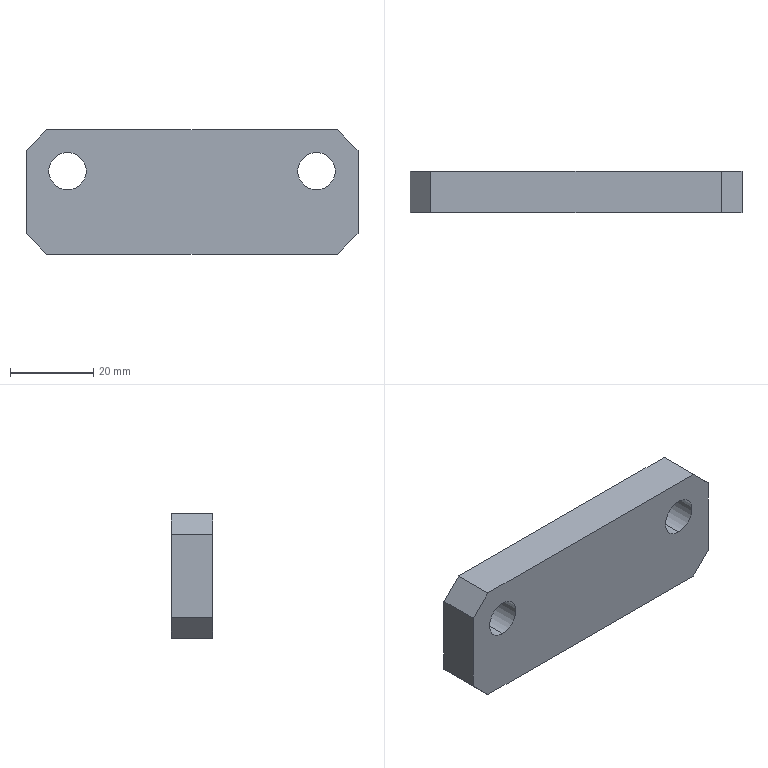Part | SolidWorks | features BaseBody 1 | 1 solid | 28 faces | box 80 x 10 x 30 mm | volume 21712 mm3 | cylinder 12 | plane 12 | cone 4 | commonest cylinder face diameters 4.2 x4 5 x4 9 x4
STEP:
#1=CARTESIAN_POINT('',(-30.,0.,0.5));
#2=VERTEX_POINT('',#1);
#3=CARTESIAN_POINT('',(-30.,0.,9.5));
#4=VERTEX_POINT('',#3);
#5=CARTESIAN_POINT('',(-30.,0.,5.));
#6=DIRECTION('',(0.,1.,0.));
#7=DIRECTION('',(0.,0.,1.));
#8=AXIS2_PLACEMENT_3D('',#5,#6,#7);
#9=CIRCLE('',#8,4.5);
#10=EDGE_CURVE('',#2,#4,#9,.T.);
#11=ORIENTED_EDGE('',*,*,#10,.F.);
#12=CARTESIAN_POINT('',(-30.,10.,0.5));
#13=VERTEX_POINT('',#12);
#14=CARTESIAN_POINT('',(-30.,10.,0.5));
#15=DIRECTION('',(0.,1.,0.));
#16=VECTOR('',#15,1000.);
#17=LINE('',#14,#16);
#18=EDGE_CURVE('',#2,#13,#17,.T.);
#19=ORIENTED_EDGE('',*,*,#18,.T.);
#20=CARTESIAN_POINT('',(-30.,10.,9.5));
#21=VERTEX_POINT('',#20);
#22=CARTESIAN_POINT('',(-30.,10.,5.));
#23=DIRECTION('',(0.,1.,0.));
#24=DIRECTION('',(0.,0.,1.));
#25=AXIS2_PLACEMENT_3D('',#22,#23,#24);
#26=CIRCLE('',#25,4.5);
#27=EDGE_CURVE('',#13,#21,#26,.T.);
#28=ORIENTED_EDGE('',*,*,#27,.T.);
#29=CARTESIAN_POINT('',(-30.,10.,9.5));
#30=DIRECTION('',(0.,1.,0.));
#31=VECTOR('',#30,1000.);
#32=LINE('',#29,#31);
#33=EDGE_CURVE('',#4,#21,#32,.T.);
#34=ORIENTED_EDGE('',*,*,#33,.F.);
#35=EDGE_LOOP('',(#11,#19,#28,#34));
#36=FACE_OUTER_BOUND('',#35,.T.);
#37=CARTESIAN_POINT('',(-30.,10.,5.));
#38=DIRECTION('',(0.,1.,0.));
#39=DIRECTION('',(0.,0.,1.));
#40=AXIS2_PLACEMENT_3D('',#37,#38,#39);
#41=CYLINDRICAL_SURFACE('',#40,4.5);
#42=ADVANCED_FACE('',(#36),#41,.F.);
#43=CARTESIAN_POINT('',(30.,0.,0.5));
#44=VERTEX_POINT('',#43);
#45=CARTESIAN_POINT('',(30.,0.,9.5));
#46=VERTEX_POINT('',#45);
#47=CARTESIAN_POINT('',(30.,0.,5.));
#48=DIRECTION('',(0.,1.,0.));
#49=DIRECTION('',(0.,0.,1.));
#50=AXIS2_PLACEMENT_3D('',#47,#48,#49);
#51=CIRCLE('',#50,4.5);
#52=EDGE_CURVE('',#44,#46,#51,.T.);
#53=ORIENTED_EDGE('',*,*,#52,.F.);
#54=CARTESIAN_POINT('',(30.,10.,0.5));
#55=VERTEX_POINT('',#54);
#56=CARTESIAN_POINT('',(30.,10.,0.5));
#57=DIRECTION('',(0.,1.,0.));
#58=VECTOR('',#57,1000.);
#59=LINE('',#56,#58);
#60=EDGE_CURVE('',#44,#55,#59,.T.);
#61=ORIENTED_EDGE('',*,*,#60,.T.);
#62=CARTESIAN_POINT('',(30.,10.,9.5));
#63=VERTEX_POINT('',#62);
#64=CARTESIAN_POINT('',(30.,10.,5.));
#65=DIRECTION('',(0.,1.,0.));
#66=DIRECTION('',(0.,0.,1.));
#67=AXIS2_PLACEMENT_3D('',#64,#65,#66);
#68=CIRCLE('',#67,4.5);
#69=EDGE_CURVE('',#55,#63,#68,.T.);
#70=ORIENTED_EDGE('',*,*,#69,.T.);
#71=CARTESIAN_POINT('',(30.,10.,9.5));
#72=DIRECTION('',(0.,1.,0.));
#73=VECTOR('',#72,1000.);
#74=LINE('',#71,#73);
#75=EDGE_CURVE('',#46,#63,#74,.T.);
#76=ORIENTED_EDGE('',*,*,#75,.F.);
#77=EDGE_LOOP('',(#53,#61,#70,#76));
#78=FACE_OUTER_BOUND('',#77,.T.);
#79=CARTESIAN_POINT('',(30.,10.,5.));
#80=DIRECTION('',(0.,1.,0.));
#81=DIRECTION('',(0.,0.,1.));
#82=AXIS2_PLACEMENT_3D('',#79,#80,#81);
#83=CYLINDRICAL_SURFACE('',#82,4.5);
#84=ADVANCED_FACE('',(#78),#83,.F.);
#85=CARTESIAN_POINT('',(17.5,5.,-5.));
#86=VERTEX_POINT('',#85);
#87=CARTESIAN_POINT('',(12.5,5.,-5.));
#88=VERTEX_POINT('',#87);
#89=CARTESIAN_POINT('',(15.,5.,-5.));
#90=DIRECTION('',(0.,0.,-1.));
#91=DIRECTION('',(-1.,0.,0.));
#92=AXIS2_PLACEMENT_3D('',#89,#90,#91);
#93=CIRCLE('',#92,2.5);
#94=EDGE_CURVE('',#86,#88,#93,.T.);
#95=ORIENTED_EDGE('',*,*,#94,.F.);
#96=CARTESIAN_POINT('',(17.5,5.,-15.));
#97=VERTEX_POINT('',#96);
#98=CARTESIAN_POINT('',(17.5,5.,-15.));
#99=DIRECTION('',(0.,0.,-1.));
#100=VECTOR('',#99,1000.);
#101=LINE('',#98,#100);
#102=EDGE_CURVE('',#86,#97,#101,.T.);
#103=ORIENTED_EDGE('',*,*,#102,.T.);
#104=CARTESIAN_POINT('',(12.5,5.,-15.));
#105=VERTEX_POINT('',#104);
#106=CARTESIAN_POINT('',(15.,5.,-15.));
#107=DIRECTION('',(0.,0.,-1.));
#108=DIRECTION('',(-1.,0.,0.));
#109=AXIS2_PLACEMENT_3D('',#106,#107,#108);
#110=CIRCLE('',#109,2.5);
#111=EDGE_CURVE('',#97,#105,#110,.T.);
#112=ORIENTED_EDGE('',*,*,#111,.T.);
#113=CARTESIAN_POINT('',(12.5,5.,-15.));
#114=DIRECTION('',(0.,0.,-1.));
#115=VECTOR('',#114,1000.);
#116=LINE('',#113,#115);
#117=EDGE_CURVE('',#88,#105,#116,.T.);
#118=ORIENTED_EDGE('',*,*,#117,.F.);
#119=EDGE_LOOP('',(#95,#103,#112,#118));
#120=FACE_OUTER_BOUND('',#119,.T.);
#121=CARTESIAN_POINT('',(15.,5.,-15.));
#122=DIRECTION('',(0.,0.,-1.));
#123=DIRECTION('',(-1.,0.,0.));
#124=AXIS2_PLACEMENT_3D('',#121,#122,#123);
#125=CYLINDRICAL_SURFACE('',#124,2.5);
#126=ADVANCED_FACE('',(#120),#125,.F.);
#127=CARTESIAN_POINT('',(17.1,5.,-1.));
#128=VERTEX_POINT('',#127);
#129=CARTESIAN_POINT('',(12.9,5.,-1.));
#130=VERTEX_POINT('',#129);
#131=CARTESIAN_POINT('',(15.,5.,-1.));
#132=DIRECTION('',(0.,0.,-1.));
#133=DIRECTION('',(-1.,0.,0.));
#134=AXIS2_PLACEMENT_3D('',#131,#132,#133);
#135=CIRCLE('',#134,2.1);
#136=EDGE_CURVE('',#128,#130,#135,.T.);
#137=ORIENTED_EDGE('',*,*,#136,.F.);
#138=CARTESIAN_POINT('',(17.1,5.,-5.));
#139=VERTEX_POINT('',#138);
#140=CARTESIAN_POINT('',(17.1,5.,-15.));
#141=DIRECTION('',(0.,0.,-1.));
#142=VECTOR('',#141,1000.);
#143=LINE('',#140,#142);
#144=EDGE_CURVE('',#128,#139,#143,.T.);
#145=ORIENTED_EDGE('',*,*,#144,.T.);
#146=CARTESIAN_POINT('',(12.9,5.,-5.));
#147=VERTEX_POINT('',#146);
#148=CARTESIAN_POINT('',(15.,5.,-5.));
#149=DIRECTION('',(0.,0.,-1.));
#150=DIRECTION('',(-1.,0.,0.));
#151=AXIS2_PLACEMENT_3D('',#148,#149,#150);
#152=CIRCLE('',#151,2.1);
#153=EDGE_CURVE('',#139,#147,#152,.T.);
#154=ORIENTED_EDGE('',*,*,#153,.T.);
#155=CARTESIAN_POINT('',(12.9,5.,-15.));
#156=DIRECTION('',(0.,0.,-1.));
#157=VECTOR('',#156,1000.);
#158=LINE('',#155,#157);
#159=EDGE_CURVE('',#130,#147,#158,.T.);
#160=ORIENTED_EDGE('',*,*,#159,.F.);
#161=EDGE_LOOP('',(#137,#145,#154,#160));
#162=FACE_OUTER_BOUND('',#161,.T.);
#163=CARTESIAN_POINT('',(15.,5.,-15.));
#164=DIRECTION('',(0.,0.,-1.));
#165=DIRECTION('',(-1.,0.,0.));
#166=AXIS2_PLACEMENT_3D('',#163,#164,#165);
#167=CYLINDRICAL_SURFACE('',#166,2.1);
#168=ADVANCED_FACE('',(#162),#167,.F.);
#169=CARTESIAN_POINT('',(15.,5.,0.2618));
#170=VERTEX_POINT('',#169);
#171=CARTESIAN_POINT('',(12.9,5.,-1.));
#172=DIRECTION('',(-0.8572,0.,-0.515));
#173=VECTOR('',#172,1000.);
#174=LINE('',#171,#173);
#175=EDGE_CURVE('',#170,#130,#174,.T.);
#176=ORIENTED_EDGE('',*,*,#175,.F.);
#177=CARTESIAN_POINT('',(17.1,5.,-1.));
#178=DIRECTION('',(0.8572,0.,-0.515));
#179=VECTOR('',#178,1000.);
#180=LINE('',#177,#179);
#181=EDGE_CURVE('',#170,#128,#180,.T.);
#182=ORIENTED_EDGE('',*,*,#181,.T.);
#183=ORIENTED_EDGE('',*,*,#136,.T.);
#184=EDGE_LOOP('',(#176,#182,#183));
#185=FACE_OUTER_BOUND('',#184,.T.);
#186=CARTESIAN_POINT('',(15.,5.,-1.));
#187=DIRECTION('',(0.,0.,-1.));
#188=DIRECTION('',(-1.,0.,0.));
#189=AXIS2_PLACEMENT_3D('',#186,#187,#188);
#190=CONICAL_SURFACE('',#189,2.1,1.03);
#191=ADVANCED_FACE('',(#185),#190,.F.);
#192=CARTESIAN_POINT('',(-12.5,5.,-5.));
#193=VERTEX_POINT('',#192);
#194=CARTESIAN_POINT('',(-17.5,5.,-5.));
#195=VERTEX_POINT('',#194);
#196=CARTESIAN_POINT('',(-15.,5.,-5.));
#197=DIRECTION('',(0.,0.,-1.));
#198=DIRECTION('',(-1.,0.,0.));
#199=AXIS2_PLACEMENT_3D('',#196,#197,#198);
#200=CIRCLE('',#199,2.5);
#201=EDGE_CURVE('',#193,#195,#200,.T.);
#202=ORIENTED_EDGE('',*,*,#201,.F.);
#203=CARTESIAN_POINT('',(-12.5,5.,-15.));
#204=VERTEX_POINT('',#203);
#205=CARTESIAN_POINT('',(-12.5,5.,-15.));
#206=DIRECTION('',(0.,0.,-1.));
#207=VECTOR('',#206,1000.);
#208=LINE('',#205,#207);
#209=EDGE_CURVE('',#193,#204,#208,.T.);
#210=ORIENTED_EDGE('',*,*,#209,.T.);
#211=CARTESIAN_POINT('',(-17.5,5.,-15.));
#212=VERTEX_POINT('',#211);
#213=CARTESIAN_POINT('',(-15.,5.,-15.));
#214=DIRECTION('',(0.,0.,-1.));
#215=DIRECTION('',(-1.,0.,0.));
#216=AXIS2_PLACEMENT_3D('',#213,#214,#215);
#217=CIRCLE('',#216,2.5);
#218=EDGE_CURVE('',#204,#212,#217,.T.);
#219=ORIENTED_EDGE('',*,*,#218,.T.);
#220=CARTESIAN_POINT('',(-17.5,5.,-15.));
#221=DIRECTION('',(0.,0.,-1.));
#222=VECTOR('',#221,1000.);
#223=LINE('',#220,#222);
#224=EDGE_CURVE('',#195,#212,#223,.T.);
#225=ORIENTED_EDGE('',*,*,#224,.F.);
#226=EDGE_LOOP('',(#202,#210,#219,#225));
#227=FACE_OUTER_BOUND('',#226,.T.);
#228=CARTESIAN_POINT('',(-15.,5.,-15.));
#229=DIRECTION('',(0.,0.,-1.));
#230=DIRECTION('',(-1.,0.,0.));
#231=AXIS2_PLACEMENT_3D('',#228,#229,#230);
#232=CYLINDRICAL_SURFACE('',#231,2.5);
#233=ADVANCED_FACE('',(#227),#232,.F.);
#234=CARTESIAN_POINT('',(-12.9,5.,-1.));
#235=VERTEX_POINT('',#234);
#236=CARTESIAN_POINT('',(-17.1,5.,-1.));
#237=VERTEX_POINT('',#236);
#238=CARTESIAN_POINT('',(-15.,5.,-1.));
#239=DIRECTION('',(0.,0.,-1.));
#240=DIRECTION('',(-1.,0.,0.));
#241=AXIS2_PLACEMENT_3D('',#238,#239,#240);
#242=CIRCLE('',#241,2.1);
#243=EDGE_CURVE('',#235,#237,#242,.T.);
#244=ORIENTED_EDGE('',*,*,#243,.F.);
#245=CARTESIAN_POINT('',(-12.9,5.,-5.));
#246=VERTEX_POINT('',#245);
#247=CARTESIAN_POINT('',(-12.9,5.,-15.));
#248=DIRECTION('',(0.,0.,-1.));
#249=VECTOR('',#248,1000.);
#250=LINE('',#247,#249);
#251=EDGE_CURVE('',#235,#246,#250,.T.);
#252=ORIENTED_EDGE('',*,*,#251,.T.);
#253=CARTESIAN_POINT('',(-17.1,5.,-5.));
#254=VERTEX_POINT('',#253);
#255=CARTESIAN_POINT('',(-15.,5.,-5.));
#256=DIRECTION('',(0.,0.,-1.));
#257=DIRECTION('',(-1.,0.,0.));
#258=AXIS2_PLACEMENT_3D('',#255,#256,#257);
#259=CIRCLE('',#258,2.1);
#260=EDGE_CURVE('',#246,#254,#259,.T.);
#261=ORIENTED_EDGE('',*,*,#260,.T.);
#262=CARTESIAN_POINT('',(-17.1,5.,-15.));
#263=DIRECTION('',(0.,0.,-1.));
#264=VECTOR('',#263,1000.);
#265=LINE('',#262,#264);
#266=EDGE_CURVE('',#237,#254,#265,.T.);
#267=ORIENTED_EDGE('',*,*,#266,.F.);
#268=EDGE_LOOP('',(#244,#252,#261,#267));
#269=FACE_OUTER_BOUND('',#268,.T.);
#270=CARTESIAN_POINT('',(-15.,5.,-15.));
#271=DIRECTION('',(0.,0.,-1.));
#272=DIRECTION('',(-1.,0.,0.));
#273=AXIS2_PLACEMENT_3D('',#270,#271,#272);
#274=CYLINDRICAL_SURFACE('',#273,2.1);
#275=ADVANCED_FACE('',(#269),#274,.F.);
#276=CARTESIAN_POINT('',(-15.,5.,0.2618));
#277=VERTEX_POINT('',#276);
#278=CARTESIAN_POINT('',(-17.1,5.,-1.));
#279=DIRECTION('',(-0.8572,0.,-0.515));
#280=VECTOR('',#279,1000.);
#281=LINE('',#278,#280);
#282=EDGE_CURVE('',#277,#237,#281,.T.);
#283=ORIENTED_EDGE('',*,*,#282,.F.);
#284=CARTESIAN_POINT('',(-12.9,5.,-1.));
#285=DIRECTION('',(0.8572,0.,-0.515));
#286=VECTOR('',#285,1000.);
#287=LINE('',#284,#286);
#288=EDGE_CURVE('',#277,#235,#287,.T.);
#289=ORIENTED_EDGE('',*,*,#288,.T.);
#290=ORIENTED_EDGE('',*,*,#243,.T.);
#291=EDGE_LOOP('',(#283,#289,#290));
#292=FACE_OUTER_BOUND('',#291,.T.);
#293=CARTESIAN_POINT('',(-15.,5.,-1.));
#294=DIRECTION('',(0.,0.,-1.));
#295=DIRECTION('',(-1.,0.,0.));
#296=AXIS2_PLACEMENT_3D('',#293,#294,#295);
#297=CONICAL_SURFACE('',#296,2.1,1.03);
#298=ADVANCED_FACE('',(#292),#297,.F.);
#299=CARTESIAN_POINT('',(-40.,0.,-10.));
#300=VERTEX_POINT('',#299);
#301=CARTESIAN_POINT('',(-40.,0.,10.));
#302=VERTEX_POINT('',#301);
#303=CARTESIAN_POINT('',(-40.,0.,-15.));
#304=DIRECTION('',(0.,0.,1.));
#305=VECTOR('',#304,1000.);
#306=LINE('',#303,#305);
#307=EDGE_CURVE('',#300,#302,#306,.T.);
#308=ORIENTED_EDGE('',*,*,#307,.T.);
#309=CARTESIAN_POINT('',(-40.,10.,10.));
#310=VERTEX_POINT('',#309);
#311=CARTESIAN_POINT('',(-40.,10.,10.));
#312=DIRECTION('',(0.,1.,0.));
#313=VECTOR('',#312,1000.);
#314=LINE('',#311,#313);
#315=EDGE_CURVE('',#302,#310,#314,.T.);
#316=ORIENTED_EDGE('',*,*,#315,.T.);
#317=CARTESIAN_POINT('',(-40.,10.,-10.));
#318=VERTEX_POINT('',#317);
#319=CARTESIAN_POINT('',(-40.,10.,-15.));
#320=DIRECTION('',(0.,0.,1.));
#321=VECTOR('',#320,1000.);
#322=LINE('',#319,#321);
#323=EDGE_CURVE('',#318,#310,#322,.T.);
#324=ORIENTED_EDGE('',*,*,#323,.F.);
#325=CARTESIAN_POINT('',(-40.,10.,-10.));
#326=DIRECTION('',(0.,-1.,0.));
#327=VECTOR('',#326,1000.);
#328=LINE('',#325,#327);
#329=EDGE_CURVE('',#318,#300,#328,.T.);
#330=ORIENTED_EDGE('',*,*,#329,.T.);
#331=EDGE_LOOP('',(#308,#316,#324,#330));
#332=FACE_OUTER_BOUND('',#331,.T.);
#333=CARTESIAN_POINT('',(-40.,10.,-15.));
#334=DIRECTION('',(1.,0.,0.));
#335=DIRECTION('',(0.,0.,-1.));
#336=AXIS2_PLACEMENT_3D('',#333,#334,#335);
#337=PLANE('',#336);
#338=ADVANCED_FACE('',(#332),#337,.F.);
#339=CARTESIAN_POINT('',(-35.,0.,15.));
#340=VERTEX_POINT('',#339);
#341=CARTESIAN_POINT('',(35.,0.,15.));
#342=VERTEX_POINT('',#341);
#343=CARTESIAN_POINT('',(40.,0.,15.));
#344=DIRECTION('',(1.,0.,0.));
#345=VECTOR('',#344,1000.);
#346=LINE('',#343,#345);
#347=EDGE_CURVE('',#340,#342,#346,.T.);
#348=ORIENTED_EDGE('',*,*,#347,.T.);
#349=CARTESIAN_POINT('',(35.,10.,15.));
#350=VERTEX_POINT('',#349);
#351=CARTESIAN_POINT('',(35.,10.,15.));
#352=DIRECTION('',(0.,1.,0.));
#353=VECTOR('',#352,1000.);
#354=LINE('',#351,#353);
#355=EDGE_CURVE('',#342,#350,#354,.T.);
#356=ORIENTED_EDGE('',*,*,#355,.T.);
#357=CARTESIAN_POINT('',(-35.,10.,15.));
#358=VERTEX_POINT('',#357);
#359=CARTESIAN_POINT('',(40.,10.,15.));
#360=DIRECTION('',(1.,0.,0.));
#361=VECTOR('',#360,1000.);
#362=LINE('',#359,#361);
#363=EDGE_CURVE('',#358,#350,#362,.T.);
#364=ORIENTED_EDGE('',*,*,#363,.F.);
#365=CARTESIAN_POINT('',(-35.,10.,15.));
#366=DIRECTION('',(0.,-1.,0.));
#367=VECTOR('',#366,1000.);
#368=LINE('',#365,#367);
#369=EDGE_CURVE('',#358,#340,#368,.T.);
#370=ORIENTED_EDGE('',*,*,#369,.T.);
#371=EDGE_LOOP('',(#348,#356,#364,#370));
#372=FACE_OUTER_BOUND('',#371,.T.);
#373=CARTESIAN_POINT('',(40.,10.,15.));
#374=DIRECTION('',(0.,0.,-1.));
#375=DIRECTION('',(-1.,0.,0.));
#376=AXIS2_PLACEMENT_3D('',#373,#374,#375);
#377=PLANE('',#376);
#378=ADVANCED_FACE('',(#372),#377,.F.);
#379=CARTESIAN_POINT('',(40.,0.,10.));
#380=VERTEX_POINT('',#379);
#381=CARTESIAN_POINT('',(40.,0.,-10.));
#382=VERTEX_POINT('',#381);
#383=CARTESIAN_POINT('',(40.,0.,-15.));
#384=DIRECTION('',(0.,0.,-1.));
#385=VECTOR('',#384,1000.);
#386=LINE('',#383,#385);
#387=EDGE_CURVE('',#380,#382,#386,.T.);
#388=ORIENTED_EDGE('',*,*,#387,.T.);
#389=CARTESIAN_POINT('',(40.,10.,-10.));
#390=VERTEX_POINT('',#389);
#391=CARTESIAN_POINT('',(40.,10.,-10.));
#392=DIRECTION('',(0.,1.,0.));
#393=VECTOR('',#392,1000.);
#394=LINE('',#391,#393);
#395=EDGE_CURVE('',#382,#390,#394,.T.);
#396=ORIENTED_EDGE('',*,*,#395,.T.);
#397=CARTESIAN_POINT('',(40.,10.,10.));
#398=VERTEX_POINT('',#397);
#399=CARTESIAN_POINT('',(40.,10.,-15.));
#400=DIRECTION('',(0.,0.,-1.));
#401=VECTOR('',#400,1000.);
#402=LINE('',#399,#401);
#403=EDGE_CURVE('',#398,#390,#402,.T.);
#404=ORIENTED_EDGE('',*,*,#403,.F.);
#405=CARTESIAN_POINT('',(40.,10.,10.));
#406=DIRECTION('',(0.,-1.,0.));
#407=VECTOR('',#406,1000.);
#408=LINE('',#405,#407);
#409=EDGE_CURVE('',#398,#380,#408,.T.);
#410=ORIENTED_EDGE('',*,*,#409,.T.);
#411=EDGE_LOOP('',(#388,#396,#404,#410));
#412=FACE_OUTER_BOUND('',#411,.T.);
#413=CARTESIAN_POINT('',(40.,10.,-15.));
#414=DIRECTION('',(-1.,0.,0.));
#415=DIRECTION('',(0.,0.,1.));
#416=AXIS2_PLACEMENT_3D('',#413,#414,#415);
#417=PLANE('',#416);
#418=ADVANCED_FACE('',(#412),#417,.F.);
#419=CARTESIAN_POINT('',(15.,5.,-15.));
#420=DIRECTION('',(0.,0.,-1.));
#421=DIRECTION('',(-1.,0.,0.));
#422=AXIS2_PLACEMENT_3D('',#419,#420,#421);
#423=CIRCLE('',#422,2.5);
#424=EDGE_CURVE('',#105,#97,#423,.T.);
#425=ORIENTED_EDGE('',*,*,#424,.F.);
#426=ORIENTED_EDGE('',*,*,#111,.F.);
#427=EDGE_LOOP('',(#425,#426));
#428=FACE_BOUND('',#427,.T.);
#429=CARTESIAN_POINT('',(-15.,5.,-15.));
#430=DIRECTION('',(0.,0.,-1.));
#431=DIRECTION('',(-1.,0.,0.));
#432=AXIS2_PLACEMENT_3D('',#429,#430,#431);
#433=CIRCLE('',#432,2.5);
#434=EDGE_CURVE('',#212,#204,#433,.T.);
#435=ORIENTED_EDGE('',*,*,#434,.F.);
#436=ORIENTED_EDGE('',*,*,#218,.F.);
#437=EDGE_LOOP('',(#435,#436));
#438=FACE_BOUND('',#437,.T.);
#439=CARTESIAN_POINT('',(35.,10.,-15.));
#440=VERTEX_POINT('',#439);
#441=CARTESIAN_POINT('',(-35.,10.,-15.));
#442=VERTEX_POINT('',#441);
#443=CARTESIAN_POINT('',(40.,10.,-15.));
#444=DIRECTION('',(-1.,0.,0.));
#445=VECTOR('',#444,1000.);
#446=LINE('',#443,#445);
#447=EDGE_CURVE('',#440,#442,#446,.T.);
#448=ORIENTED_EDGE('',*,*,#447,.F.);
#449=CARTESIAN_POINT('',(35.,0.,-15.));
#450=VERTEX_POINT('',#449);
#451=CARTESIAN_POINT('',(35.,10.,-15.));
#452=DIRECTION('',(0.,-1.,0.));
#453=VECTOR('',#452,1000.);
#454=LINE('',#451,#453);
#455=EDGE_CURVE('',#440,#450,#454,.T.);
#456=ORIENTED_EDGE('',*,*,#455,.T.);
#457=CARTESIAN_POINT('',(-35.,0.,-15.));
#458=VERTEX_POINT('',#457);
#459=CARTESIAN_POINT('',(40.,0.,-15.));
#460=DIRECTION('',(-1.,0.,0.));
#461=VECTOR('',#460,1000.);
#462=LINE('',#459,#461);
#463=EDGE_CURVE('',#450,#458,#462,.T.);
#464=ORIENTED_EDGE('',*,*,#463,.T.);
#465=CARTESIAN_POINT('',(-35.,10.,-15.));
#466=DIRECTION('',(0.,1.,0.));
#467=VECTOR('',#466,1000.);
#468=LINE('',#465,#467);
#469=EDGE_CURVE('',#458,#442,#468,.T.);
#470=ORIENTED_EDGE('',*,*,#469,.T.);
#471=EDGE_LOOP('',(#448,#456,#464,#470));
#472=FACE_OUTER_BOUND('',#471,.T.);
#473=CARTESIAN_POINT('',(40.,10.,-15.));
#474=DIRECTION('',(0.,0.,1.));
#475=DIRECTION('',(1.,0.,0.));
#476=AXIS2_PLACEMENT_3D('',#473,#474,#475);
#477=PLANE('',#476);
#478=ADVANCED_FACE('',(#428,#438,#472),#477,.F.);
#479=CARTESIAN_POINT('',(-30.,10.,5.));
#480=DIRECTION('',(0.,1.,0.));
#481=DIRECTION('',(0.,0.,1.));
#482=AXIS2_PLACEMENT_3D('',#479,#480,#481);
#483=CIRCLE('',#482,4.5);
#484=EDGE_CURVE('',#21,#13,#483,.T.);
#485=ORIENTED_EDGE('',*,*,#484,.F.);
#486=ORIENTED_EDGE('',*,*,#27,.F.);
#487=EDGE_LOOP('',(#485,#486));
#488=FACE_BOUND('',#487,.T.);
#489=CARTESIAN_POINT('',(30.,10.,5.));
#490=DIRECTION('',(0.,1.,0.));
#491=DIRECTION('',(0.,0.,1.));
#492=AXIS2_PLACEMENT_3D('',#489,#490,#491);
#493=CIRCLE('',#492,4.5);
#494=EDGE_CURVE('',#63,#55,#493,.T.);
#495=ORIENTED_EDGE('',*,*,#494,.F.);
#496=ORIENTED_EDGE('',*,*,#69,.F.);
#497=EDGE_LOOP('',(#495,#496));
#498=FACE_BOUND('',#497,.T.);
#499=ORIENTED_EDGE('',*,*,#403,.T.);
#500=CARTESIAN_POINT('',(35.,10.,-15.));
#501=DIRECTION('',(-0.7071,0.,-0.7071));
#502=VECTOR('',#501,1000.);
#503=LINE('',#500,#502);
#504=EDGE_CURVE('',#390,#440,#503,.T.);
#505=ORIENTED_EDGE('',*,*,#504,.T.);
#506=ORIENTED_EDGE('',*,*,#447,.T.);
#507=CARTESIAN_POINT('',(-40.,10.,-10.));
#508=DIRECTION('',(-0.7071,0.,0.7071));
#509=VECTOR('',#508,1000.);
#510=LINE('',#507,#509);
#511=EDGE_CURVE('',#442,#318,#510,.T.);
#512=ORIENTED_EDGE('',*,*,#511,.T.);
#513=ORIENTED_EDGE('',*,*,#323,.T.);
#514=CARTESIAN_POINT('',(-35.,10.,15.));
#515=DIRECTION('',(0.7071,0.,0.7071));
#516=VECTOR('',#515,1000.);
#517=LINE('',#514,#516);
#518=EDGE_CURVE('',#310,#358,#517,.T.);
#519=ORIENTED_EDGE('',*,*,#518,.T.);
#520=ORIENTED_EDGE('',*,*,#363,.T.);
#521=CARTESIAN_POINT('',(40.,10.,10.));
#522=DIRECTION('',(0.7071,0.,-0.7071));
#523=VECTOR('',#522,1000.);
#524=LINE('',#521,#523);
#525=EDGE_CURVE('',#350,#398,#524,.T.);
#526=ORIENTED_EDGE('',*,*,#525,.T.);
#527=EDGE_LOOP('',(#499,#505,#506,#512,#513,#519,#520,#526));
#528=FACE_OUTER_BOUND('',#527,.T.);
#529=CARTESIAN_POINT('',(0.,10.,0.));
#530=DIRECTION('',(0.,-1.,0.));
#531=DIRECTION('',(0.,0.,-1.));
#532=AXIS2_PLACEMENT_3D('',#529,#530,#531);
#533=PLANE('',#532);
#534=ADVANCED_FACE('',(#488,#498,#528),#533,.F.);
#535=CARTESIAN_POINT('',(-30.,0.,5.));
#536=DIRECTION('',(0.,1.,0.));
#537=DIRECTION('',(0.,0.,1.));
#538=AXIS2_PLACEMENT_3D('',#535,#536,#537);
#539=CIRCLE('',#538,4.5);
#540=EDGE_CURVE('',#4,#2,#539,.T.);
#541=ORIENTED_EDGE('',*,*,#540,.T.);
#542=ORIENTED_EDGE('',*,*,#10,.T.);
#543=EDGE_LOOP('',(#541,#542));
#544=FACE_BOUND('',#543,.T.);
#545=CARTESIAN_POINT('',(30.,0.,5.));
#546=DIRECTION('',(0.,1.,0.));
#547=DIRECTION('',(0.,0.,1.));
#548=AXIS2_PLACEMENT_3D('',#545,#546,#547);
#549=CIRCLE('',#548,4.5);
#550=EDGE_CURVE('',#46,#44,#549,.T.);
#551=ORIENTED_EDGE('',*,*,#550,.T.);
#552=ORIENTED_EDGE('',*,*,#52,.T.);
#553=EDGE_LOOP('',(#551,#552));
#554=FACE_BOUND('',#553,.T.);
#555=ORIENTED_EDGE('',*,*,#463,.F.);
#556=CARTESIAN_POINT('',(25.,0.,-25.));
#557=DIRECTION('',(0.7071,0.,0.7071));
#558=VECTOR('',#557,1000.);
#559=LINE('',#556,#558);
#560=EDGE_CURVE('',#450,#382,#559,.T.);
#561=ORIENTED_EDGE('',*,*,#560,.T.);
#562=ORIENTED_EDGE('',*,*,#387,.F.);
#563=CARTESIAN_POINT('',(25.,0.,25.));
#564=DIRECTION('',(-0.7071,0.,0.7071));
#565=VECTOR('',#564,1000.);
#566=LINE('',#563,#565);
#567=EDGE_CURVE('',#380,#342,#566,.T.);
#568=ORIENTED_EDGE('',*,*,#567,.T.);
#569=ORIENTED_EDGE('',*,*,#347,.F.);
#570=CARTESIAN_POINT('',(-25.,0.,25.));
#571=DIRECTION('',(-0.7071,0.,-0.7071));
#572=VECTOR('',#571,1000.);
#573=LINE('',#570,#572);
#574=EDGE_CURVE('',#340,#302,#573,.T.);
#575=ORIENTED_EDGE('',*,*,#574,.T.);
#576=ORIENTED_EDGE('',*,*,#307,.F.);
#577=CARTESIAN_POINT('',(-25.,0.,-25.));
#578=DIRECTION('',(0.7071,0.,-0.7071));
#579=VECTOR('',#578,1000.);
#580=LINE('',#577,#579);
#581=EDGE_CURVE('',#300,#458,#580,.T.);
#582=ORIENTED_EDGE('',*,*,#581,.T.);
#583=EDGE_LOOP('',(#555,#561,#562,#568,#569,#575,#576,#582));
#584=FACE_OUTER_BOUND('',#583,.T.);
#585=CARTESIAN_POINT('',(0.,0.,0.));
#586=DIRECTION('',(0.,-1.,0.));
#587=DIRECTION('',(0.,0.,-1.));
#588=AXIS2_PLACEMENT_3D('',#585,#586,#587);
#589=PLANE('',#588);
#590=ADVANCED_FACE('',(#544,#554,#584),#589,.T.);
#591=ORIENTED_EDGE('',*,*,#288,.F.);
#592=ORIENTED_EDGE('',*,*,#282,.T.);
#593=CARTESIAN_POINT('',(-15.,5.,-1.));
#594=DIRECTION('',(0.,0.,-1.));
#595=DIRECTION('',(-1.,0.,0.));
#596=AXIS2_PLACEMENT_3D('',#593,#594,#595);
#597=CIRCLE('',#596,2.1);
#598=EDGE_CURVE('',#237,#235,#597,.T.);
#599=ORIENTED_EDGE('',*,*,#598,.T.);
#600=EDGE_LOOP('',(#591,#592,#599));
#601=FACE_OUTER_BOUND('',#600,.T.);
#602=CARTESIAN_POINT('',(-15.,5.,-1.));
#603=DIRECTION('',(0.,0.,-1.));
#604=DIRECTION('',(-1.,0.,0.));
#605=AXIS2_PLACEMENT_3D('',#602,#603,#604);
#606=CONICAL_SURFACE('',#605,2.1,1.03);
#607=ADVANCED_FACE('',(#601),#606,.F.);
#608=ORIENTED_EDGE('',*,*,#251,.F.);
#609=ORIENTED_EDGE('',*,*,#598,.F.);
#610=ORIENTED_EDGE('',*,*,#266,.T.);
#611=CARTESIAN_POINT('',(-15.,5.,-5.));
#612=DIRECTION('',(0.,0.,-1.));
#613=DIRECTION('',(-1.,0.,0.));
#614=AXIS2_PLACEMENT_3D('',#611,#612,#613);
#615=CIRCLE('',#614,2.1);
#616=EDGE_CURVE('',#254,#246,#615,.T.);
#617=ORIENTED_EDGE('',*,*,#616,.T.);
#618=EDGE_LOOP('',(#608,#609,#610,#617));
#619=FACE_OUTER_BOUND('',#618,.T.);
#620=CARTESIAN_POINT('',(-15.,5.,-15.));
#621=DIRECTION('',(0.,0.,-1.));
#622=DIRECTION('',(-1.,0.,0.));
#623=AXIS2_PLACEMENT_3D('',#620,#621,#622);
#624=CYLINDRICAL_SURFACE('',#623,2.1);
#625=ADVANCED_FACE('',(#619),#624,.F.);
#626=ORIENTED_EDGE('',*,*,#616,.F.);
#627=ORIENTED_EDGE('',*,*,#260,.F.);
#628=EDGE_LOOP('',(#626,#627));
#629=FACE_BOUND('',#628,.T.);
#630=CARTESIAN_POINT('',(-15.,5.,-5.));
#631=DIRECTION('',(0.,0.,-1.));
#632=DIRECTION('',(-1.,0.,0.));
#633=AXIS2_PLACEMENT_3D('',#630,#631,#632);
#634=CIRCLE('',#633,2.5);
#635=EDGE_CURVE('',#195,#193,#634,.T.);
#636=ORIENTED_EDGE('',*,*,#635,.T.);
#637=ORIENTED_EDGE('',*,*,#201,.T.);
#638=EDGE_LOOP('',(#636,#637));
#639=FACE_OUTER_BOUND('',#638,.T.);
#640=CARTESIAN_POINT('',(-12.9,5.,-5.));
#641=DIRECTION('',(0.,0.,1.));
#642=DIRECTION('',(1.,0.,0.));
#643=AXIS2_PLACEMENT_3D('',#640,#641,#642);
#644=PLANE('',#643);
#645=ADVANCED_FACE('',(#629,#639),#644,.F.);
#646=ORIENTED_EDGE('',*,*,#209,.F.);
#647=ORIENTED_EDGE('',*,*,#635,.F.);
#648=ORIENTED_EDGE('',*,*,#224,.T.);
#649=ORIENTED_EDGE('',*,*,#434,.T.);
#650=EDGE_LOOP('',(#646,#647,#648,#649));
#651=FACE_OUTER_BOUND('',#650,.T.);
#652=CARTESIAN_POINT('',(-15.,5.,-15.));
#653=DIRECTION('',(0.,0.,-1.));
#654=DIRECTION('',(-1.,0.,0.));
#655=AXIS2_PLACEMENT_3D('',#652,#653,#654);
#656=CYLINDRICAL_SURFACE('',#655,2.5);
#657=ADVANCED_FACE('',(#651),#656,.F.);
#658=ORIENTED_EDGE('',*,*,#181,.F.);
#659=ORIENTED_EDGE('',*,*,#175,.T.);
#660=CARTESIAN_POINT('',(15.,5.,-1.));
#661=DIRECTION('',(0.,0.,-1.));
#662=DIRECTION('',(-1.,0.,0.));
#663=AXIS2_PLACEMENT_3D('',#660,#661,#662);
#664=CIRCLE('',#663,2.1);
#665=EDGE_CURVE('',#130,#128,#664,.T.);
#666=ORIENTED_EDGE('',*,*,#665,.T.);
#667=EDGE_LOOP('',(#658,#659,#666));
#668=FACE_OUTER_BOUND('',#667,.T.);
#669=CARTESIAN_POINT('',(15.,5.,-1.));
#670=DIRECTION('',(0.,0.,-1.));
#671=DIRECTION('',(-1.,0.,0.));
#672=AXIS2_PLACEMENT_3D('',#669,#670,#671);
#673=CONICAL_SURFACE('',#672,2.1,1.03);
#674=ADVANCED_FACE('',(#668),#673,.F.);
#675=ORIENTED_EDGE('',*,*,#144,.F.);
#676=ORIENTED_EDGE('',*,*,#665,.F.);
#677=ORIENTED_EDGE('',*,*,#159,.T.);
#678=CARTESIAN_POINT('',(15.,5.,-5.));
#679=DIRECTION('',(0.,0.,-1.));
#680=DIRECTION('',(-1.,0.,0.));
#681=AXIS2_PLACEMENT_3D('',#678,#679,#680);
#682=CIRCLE('',#681,2.1);
#683=EDGE_CURVE('',#147,#139,#682,.T.);
#684=ORIENTED_EDGE('',*,*,#683,.T.);
#685=EDGE_LOOP('',(#675,#676,#677,#684));
#686=FACE_OUTER_BOUND('',#685,.T.);
#687=CARTESIAN_POINT('',(15.,5.,-15.));
#688=DIRECTION('',(0.,0.,-1.));
#689=DIRECTION('',(-1.,0.,0.));
#690=AXIS2_PLACEMENT_3D('',#687,#688,#689);
#691=CYLINDRICAL_SURFACE('',#690,2.1);
#692=ADVANCED_FACE('',(#686),#691,.F.);
#693=ORIENTED_EDGE('',*,*,#683,.F.);
#694=ORIENTED_EDGE('',*,*,#153,.F.);
#695=EDGE_LOOP('',(#693,#694));
#696=FACE_BOUND('',#695,.T.);
#697=CARTESIAN_POINT('',(15.,5.,-5.));
#698=DIRECTION('',(0.,0.,-1.));
#699=DIRECTION('',(-1.,0.,0.));
#700=AXIS2_PLACEMENT_3D('',#697,#698,#699);
#701=CIRCLE('',#700,2.5);
#702=EDGE_CURVE('',#88,#86,#701,.T.);
#703=ORIENTED_EDGE('',*,*,#702,.T.);
#704=ORIENTED_EDGE('',*,*,#94,.T.);
#705=EDGE_LOOP('',(#703,#704));
#706=FACE_OUTER_BOUND('',#705,.T.);
#707=CARTESIAN_POINT('',(17.1,5.,-5.));
#708=DIRECTION('',(0.,0.,1.));
#709=DIRECTION('',(1.,0.,0.));
#710=AXIS2_PLACEMENT_3D('',#707,#708,#709);
#711=PLANE('',#710);
#712=ADVANCED_FACE('',(#696,#706),#711,.F.);
#713=ORIENTED_EDGE('',*,*,#102,.F.);
#714=ORIENTED_EDGE('',*,*,#702,.F.);
#715=ORIENTED_EDGE('',*,*,#117,.T.);
#716=ORIENTED_EDGE('',*,*,#424,.T.);
#717=EDGE_LOOP('',(#713,#714,#715,#716));
#718=FACE_OUTER_BOUND('',#717,.T.);
#719=CARTESIAN_POINT('',(15.,5.,-15.));
#720=DIRECTION('',(0.,0.,-1.));
#721=DIRECTION('',(-1.,0.,0.));
#722=AXIS2_PLACEMENT_3D('',#719,#720,#721);
#723=CYLINDRICAL_SURFACE('',#722,2.5);
#724=ADVANCED_FACE('',(#718),#723,.F.);
#725=ORIENTED_EDGE('',*,*,#504,.F.);
#726=ORIENTED_EDGE('',*,*,#395,.F.);
#727=ORIENTED_EDGE('',*,*,#560,.F.);
#728=ORIENTED_EDGE('',*,*,#455,.F.);
#729=EDGE_LOOP('',(#725,#726,#727,#728));
#730=FACE_OUTER_BOUND('',#729,.T.);
#731=CARTESIAN_POINT('',(35.,10.,-15.));
#732=DIRECTION('',(-0.7071,0.,0.7071));
#733=DIRECTION('',(0.,-1.,0.));
#734=AXIS2_PLACEMENT_3D('',#731,#732,#733);
#735=PLANE('',#734);
#736=ADVANCED_FACE('',(#730),#735,.F.);
#737=ORIENTED_EDGE('',*,*,#525,.F.);
#738=ORIENTED_EDGE('',*,*,#355,.F.);
#739=ORIENTED_EDGE('',*,*,#567,.F.);
#740=ORIENTED_EDGE('',*,*,#409,.F.);
#741=EDGE_LOOP('',(#737,#738,#739,#740));
#742=FACE_OUTER_BOUND('',#741,.T.);
#743=CARTESIAN_POINT('',(40.,10.,10.));
#744=DIRECTION('',(-0.7071,0.,-0.7071));
#745=DIRECTION('',(0.,-1.,0.));
#746=AXIS2_PLACEMENT_3D('',#743,#744,#745);
#747=PLANE('',#746);
#748=ADVANCED_FACE('',(#742),#747,.F.);
#749=ORIENTED_EDGE('',*,*,#518,.F.);
#750=ORIENTED_EDGE('',*,*,#315,.F.);
#751=ORIENTED_EDGE('',*,*,#574,.F.);
#752=ORIENTED_EDGE('',*,*,#369,.F.);
#753=EDGE_LOOP('',(#749,#750,#751,#752));
#754=FACE_OUTER_BOUND('',#753,.T.);
#755=CARTESIAN_POINT('',(-35.,10.,15.));
#756=DIRECTION('',(0.7071,0.,-0.7071));
#757=DIRECTION('',(0.,-1.,0.));
#758=AXIS2_PLACEMENT_3D('',#755,#756,#757);
#759=PLANE('',#758);
#760=ADVANCED_FACE('',(#754),#759,.F.);
#761=ORIENTED_EDGE('',*,*,#511,.F.);
#762=ORIENTED_EDGE('',*,*,#469,.F.);
#763=ORIENTED_EDGE('',*,*,#581,.F.);
#764=ORIENTED_EDGE('',*,*,#329,.F.);
#765=EDGE_LOOP('',(#761,#762,#763,#764));
#766=FACE_OUTER_BOUND('',#765,.T.);
#767=CARTESIAN_POINT('',(-40.,10.,-10.));
#768=DIRECTION('',(0.7071,0.,0.7071));
#769=DIRECTION('',(0.,-1.,0.));
#770=AXIS2_PLACEMENT_3D('',#767,#768,#769);
#771=PLANE('',#770);
#772=ADVANCED_FACE('',(#766),#771,.F.);
#773=ORIENTED_EDGE('',*,*,#60,.F.);
#774=ORIENTED_EDGE('',*,*,#550,.F.);
#775=ORIENTED_EDGE('',*,*,#75,.T.);
#776=ORIENTED_EDGE('',*,*,#494,.T.);
#777=EDGE_LOOP('',(#773,#774,#775,#776));
#778=FACE_OUTER_BOUND('',#777,.T.);
#779=CARTESIAN_POINT('',(30.,10.,5.));
#780=DIRECTION('',(0.,1.,0.));
#781=DIRECTION('',(0.,0.,1.));
#782=AXIS2_PLACEMENT_3D('',#779,#780,#781);
#783=CYLINDRICAL_SURFACE('',#782,4.5);
#784=ADVANCED_FACE('',(#778),#783,.F.);
#785=ORIENTED_EDGE('',*,*,#18,.F.);
#786=ORIENTED_EDGE('',*,*,#540,.F.);
#787=ORIENTED_EDGE('',*,*,#33,.T.);
#788=ORIENTED_EDGE('',*,*,#484,.T.);
#789=EDGE_LOOP('',(#785,#786,#787,#788));
#790=FACE_OUTER_BOUND('',#789,.T.);
#791=CARTESIAN_POINT('',(-30.,10.,5.));
#792=DIRECTION('',(0.,1.,0.));
#793=DIRECTION('',(0.,0.,1.));
#794=AXIS2_PLACEMENT_3D('',#791,#792,#793);
#795=CYLINDRICAL_SURFACE('',#794,4.5);
#796=ADVANCED_FACE('',(#790),#795,.F.);
#797=CLOSED_SHELL('',(#42,#84,#126,#168,#191,#233,#275,#298,#338,#378,#418,#478,#534,#590,#607,#625,#645,#657,#674,#692,#712,#724,#736,#748,#760,#772,#784,#796));
#798=MANIFOLD_SOLID_BREP('',#797);
#799=CARTESIAN_POINT('',(0.,0.,0.));
#800=DIRECTION('',(0.,0.,1.));
#801=DIRECTION('',(1.,0.,0.));
#802=AXIS2_PLACEMENT_3D('',#799,#800,#801);
#803=(LENGTH_UNIT()NAMED_UNIT(*)SI_UNIT(.MILLI.,.METRE.));
#804=UNCERTAINTY_MEASURE_WITH_UNIT(LENGTH_MEASURE(0.00001),#803,'','');
#805=(NAMED_UNIT(*)PLANE_ANGLE_UNIT()SI_UNIT($,.RADIAN.));
#806=(NAMED_UNIT(*)SI_UNIT($,.STERADIAN.)SOLID_ANGLE_UNIT());
#807=(GEOMETRIC_REPRESENTATION_CONTEXT(3)GLOBAL_UNCERTAINTY_ASSIGNED_CONTEXT((#804))GLOBAL_UNIT_ASSIGNED_CONTEXT((#803,#805,#806))REPRESENTATION_CONTEXT('',''));
#808=ADVANCED_BREP_SHAPE_REPRESENTATION('',(#798,#802),#807);